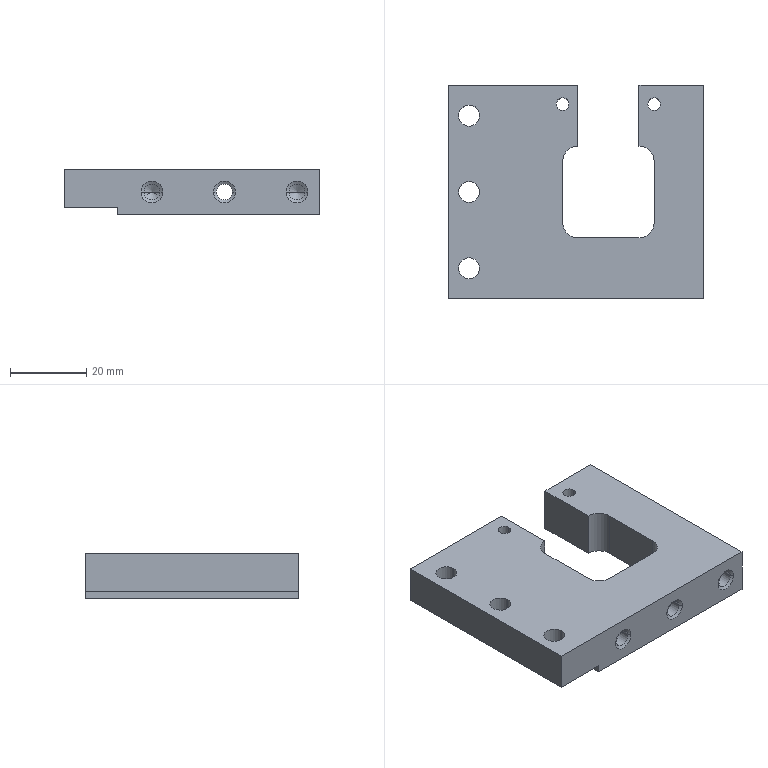Part | NX | 1 solid | 48 faces | box 67 x 56 x 12 mm | volume 32065 mm3 | cylinder 20 | plane 14 | cone 14 | commonest cylinder face diameters 4.2 x6 5.5 x6 3.3 x4 8 x4
STEP:
#1=CARTESIAN_POINT('',(480.1,203.33,-200.53));
#2=VERTEX_POINT('',#1);
#3=CARTESIAN_POINT('',(497.1,203.33,-200.53));
#4=VERTEX_POINT('',#3);
#5=CARTESIAN_POINT('',(435.607,203.33,-200.53));
#6=DIRECTION('',(1.,0.,0.));
#7=VECTOR('',#6,1000.);
#8=LINE('',#5,#7);
#9=EDGE_CURVE('',#2,#4,#8,.T.);
#10=ORIENTED_EDGE('',*,*,#9,.F.);
#11=CARTESIAN_POINT('',(480.1,203.33,-188.53));
#12=VERTEX_POINT('',#11);
#13=CARTESIAN_POINT('',(480.1,203.33,-198.53));
#14=DIRECTION('',(0.,0.,1.));
#15=VECTOR('',#14,1000.);
#16=LINE('',#13,#15);
#17=EDGE_CURVE('',#2,#12,#16,.T.);
#18=ORIENTED_EDGE('',*,*,#17,.T.);
#19=CARTESIAN_POINT('',(497.1,203.33,-188.53));
#20=VERTEX_POINT('',#19);
#21=CARTESIAN_POINT('',(435.607,203.33,-188.53));
#22=DIRECTION('',(-1.,0.,0.));
#23=VECTOR('',#22,1000.);
#24=LINE('',#21,#23);
#25=EDGE_CURVE('',#20,#12,#24,.T.);
#26=ORIENTED_EDGE('',*,*,#25,.F.);
#27=CARTESIAN_POINT('',(497.1,203.33,-198.53));
#28=DIRECTION('',(0.,0.,1.));
#29=VECTOR('',#28,1000.);
#30=LINE('',#27,#29);
#31=EDGE_CURVE('',#4,#20,#30,.T.);
#32=ORIENTED_EDGE('',*,*,#31,.F.);
#33=EDGE_LOOP('',(#10,#18,#26,#32));
#34=FACE_BOUND('',#33,.T.);
#35=CARTESIAN_POINT('',(430.1,203.33,-198.53));
#36=DIRECTION('',(0.,1.,0.));
#37=DIRECTION('',(1.,0.,0.));
#38=AXIS2_PLACEMENT_3D('',#35,#36,#37);
#39=PLANE('',#38);
#40=ADVANCED_FACE('',(#34),#39,.T.);
#41=CARTESIAN_POINT('',(430.1,147.33,-198.53));
#42=VERTEX_POINT('',#41);
#43=CARTESIAN_POINT('',(444.1,147.33,-198.53));
#44=VERTEX_POINT('',#43);
#45=CARTESIAN_POINT('',(435.607,147.33,-198.53));
#46=DIRECTION('',(1.,0.,0.));
#47=VECTOR('',#46,1000.);
#48=LINE('',#45,#47);
#49=EDGE_CURVE('',#42,#44,#48,.T.);
#50=ORIENTED_EDGE('',*,*,#49,.T.);
#51=CARTESIAN_POINT('',(444.1,147.33,-200.53));
#52=VERTEX_POINT('',#51);
#53=CARTESIAN_POINT('',(444.1,147.33,-198.53));
#54=DIRECTION('',(0.,0.,1.));
#55=VECTOR('',#54,1000.);
#56=LINE('',#53,#55);
#57=EDGE_CURVE('',#52,#44,#56,.T.);
#58=ORIENTED_EDGE('',*,*,#57,.F.);
#59=CARTESIAN_POINT('',(497.1,147.33,-200.53));
#60=VERTEX_POINT('',#59);
#61=CARTESIAN_POINT('',(435.607,147.33,-200.53));
#62=DIRECTION('',(-1.,0.,0.));
#63=VECTOR('',#62,1000.);
#64=LINE('',#61,#63);
#65=EDGE_CURVE('',#60,#52,#64,.T.);
#66=ORIENTED_EDGE('',*,*,#65,.F.);
#67=CARTESIAN_POINT('',(497.1,147.33,-188.53));
#68=VERTEX_POINT('',#67);
#69=CARTESIAN_POINT('',(497.1,147.33,-198.53));
#70=DIRECTION('',(0.,0.,1.));
#71=VECTOR('',#70,1000.);
#72=LINE('',#69,#71);
#73=EDGE_CURVE('',#60,#68,#72,.T.);
#74=ORIENTED_EDGE('',*,*,#73,.T.);
#75=CARTESIAN_POINT('',(430.1,147.33,-188.53));
#76=VERTEX_POINT('',#75);
#77=CARTESIAN_POINT('',(435.607,147.33,-188.53));
#78=DIRECTION('',(1.,0.,0.));
#79=VECTOR('',#78,1000.);
#80=LINE('',#77,#79);
#81=EDGE_CURVE('',#76,#68,#80,.T.);
#82=ORIENTED_EDGE('',*,*,#81,.F.);
#83=CARTESIAN_POINT('',(430.1,147.33,-198.53));
#84=DIRECTION('',(0.,0.,-1.));
#85=VECTOR('',#84,1000.);
#86=LINE('',#83,#85);
#87=EDGE_CURVE('',#76,#42,#86,.T.);
#88=ORIENTED_EDGE('',*,*,#87,.T.);
#89=EDGE_LOOP('',(#50,#58,#66,#74,#82,#88));
#90=FACE_BOUND('',#89,.T.);
#91=CARTESIAN_POINT('',(469.24,147.33,-194.53));
#92=VERTEX_POINT('',#91);
#93=CARTESIAN_POINT('',(474.96,147.33,-194.53));
#94=VERTEX_POINT('',#93);
#95=CARTESIAN_POINT('',(472.1,147.33,-194.53));
#96=DIRECTION('',(0.,-1.,0.));
#97=DIRECTION('',(-1.,0.,0.));
#98=AXIS2_PLACEMENT_3D('',#95,#96,#97);
#99=CIRCLE('',#98,2.86);
#100=EDGE_CURVE('',#92,#94,#99,.T.);
#101=ORIENTED_EDGE('',*,*,#100,.F.);
#102=CARTESIAN_POINT('',(472.1,147.33,-194.53));
#103=DIRECTION('',(0.,-1.,0.));
#104=DIRECTION('',(-1.,0.,0.));
#105=AXIS2_PLACEMENT_3D('',#102,#103,#104);
#106=CIRCLE('',#105,2.86);
#107=EDGE_CURVE('',#94,#92,#106,.T.);
#108=ORIENTED_EDGE('',*,*,#107,.F.);
#109=EDGE_LOOP('',(#101,#108));
#110=FACE_BOUND('',#109,.T.);
#111=CARTESIAN_POINT('',(455.96,147.33,-194.53));
#112=VERTEX_POINT('',#111);
#113=CARTESIAN_POINT('',(450.24,147.33,-194.53));
#114=VERTEX_POINT('',#113);
#115=CARTESIAN_POINT('',(453.1,147.33,-194.53));
#116=DIRECTION('',(0.,-1.,0.));
#117=DIRECTION('',(-1.,0.,0.));
#118=AXIS2_PLACEMENT_3D('',#115,#116,#117);
#119=CIRCLE('',#118,2.86);
#120=EDGE_CURVE('',#112,#114,#119,.T.);
#121=ORIENTED_EDGE('',*,*,#120,.F.);
#122=CARTESIAN_POINT('',(453.1,147.33,-194.53));
#123=DIRECTION('',(0.,-1.,0.));
#124=DIRECTION('',(-1.,0.,0.));
#125=AXIS2_PLACEMENT_3D('',#122,#123,#124);
#126=CIRCLE('',#125,2.86);
#127=EDGE_CURVE('',#114,#112,#126,.T.);
#128=ORIENTED_EDGE('',*,*,#127,.F.);
#129=EDGE_LOOP('',(#121,#128));
#130=FACE_BOUND('',#129,.T.);
#131=CARTESIAN_POINT('',(488.24,147.33,-194.53));
#132=VERTEX_POINT('',#131);
#133=CARTESIAN_POINT('',(493.96,147.33,-194.53));
#134=VERTEX_POINT('',#133);
#135=CARTESIAN_POINT('',(491.1,147.33,-194.53));
#136=DIRECTION('',(0.,-1.,0.));
#137=DIRECTION('',(-1.,0.,0.));
#138=AXIS2_PLACEMENT_3D('',#135,#136,#137);
#139=CIRCLE('',#138,2.86);
#140=EDGE_CURVE('',#132,#134,#139,.T.);
#141=ORIENTED_EDGE('',*,*,#140,.F.);
#142=CARTESIAN_POINT('',(491.1,147.33,-194.53));
#143=DIRECTION('',(0.,-1.,0.));
#144=DIRECTION('',(-1.,0.,0.));
#145=AXIS2_PLACEMENT_3D('',#142,#143,#144);
#146=CIRCLE('',#145,2.86);
#147=EDGE_CURVE('',#134,#132,#146,.T.);
#148=ORIENTED_EDGE('',*,*,#147,.F.);
#149=EDGE_LOOP('',(#141,#148));
#150=FACE_BOUND('',#149,.T.);
#151=CARTESIAN_POINT('',(444.1,147.33,-198.53));
#152=DIRECTION('',(0.,-1.,0.));
#153=DIRECTION('',(0.,0.,-1.));
#154=AXIS2_PLACEMENT_3D('',#151,#152,#153);
#155=PLANE('',#154);
#156=ADVANCED_FACE('',(#90,#110,#130,#150),#155,.T.);
#157=CARTESIAN_POINT('',(430.1,203.33,-198.53));
#158=VERTEX_POINT('',#157);
#159=CARTESIAN_POINT('',(430.1,236.208,-198.53));
#160=DIRECTION('',(0.,1.,0.));
#161=VECTOR('',#160,1000.);
#162=LINE('',#159,#161);
#163=EDGE_CURVE('',#42,#158,#162,.T.);
#164=ORIENTED_EDGE('',*,*,#163,.F.);
#165=ORIENTED_EDGE('',*,*,#87,.F.);
#166=CARTESIAN_POINT('',(430.1,203.33,-188.53));
#167=VERTEX_POINT('',#166);
#168=CARTESIAN_POINT('',(430.1,236.208,-188.53));
#169=DIRECTION('',(0.,-1.,0.));
#170=VECTOR('',#169,1000.);
#171=LINE('',#168,#170);
#172=EDGE_CURVE('',#167,#76,#171,.T.);
#173=ORIENTED_EDGE('',*,*,#172,.F.);
#174=CARTESIAN_POINT('',(430.1,203.33,-198.53));
#175=DIRECTION('',(0.,0.,-1.));
#176=VECTOR('',#175,1000.);
#177=LINE('',#174,#176);
#178=EDGE_CURVE('',#167,#158,#177,.T.);
#179=ORIENTED_EDGE('',*,*,#178,.T.);
#180=EDGE_LOOP('',(#164,#165,#173,#179));
#181=FACE_BOUND('',#180,.T.);
#182=CARTESIAN_POINT('',(430.1,145.33,-198.53));
#183=DIRECTION('',(-1.,0.,0.));
#184=DIRECTION('',(0.,0.,1.));
#185=AXIS2_PLACEMENT_3D('',#182,#183,#184);
#186=PLANE('',#185);
#187=ADVANCED_FACE('',(#181),#186,.T.);
#188=CARTESIAN_POINT('',(497.1,236.208,-200.53));
#189=DIRECTION('',(0.,-1.,0.));
#190=VECTOR('',#189,1000.);
#191=LINE('',#188,#190);
#192=EDGE_CURVE('',#4,#60,#191,.T.);
#193=ORIENTED_EDGE('',*,*,#192,.F.);
#194=ORIENTED_EDGE('',*,*,#31,.T.);
#195=CARTESIAN_POINT('',(497.1,236.208,-188.53));
#196=DIRECTION('',(0.,1.,0.));
#197=VECTOR('',#196,1000.);
#198=LINE('',#195,#197);
#199=EDGE_CURVE('',#68,#20,#198,.T.);
#200=ORIENTED_EDGE('',*,*,#199,.F.);
#201=ORIENTED_EDGE('',*,*,#73,.F.);
#202=EDGE_LOOP('',(#193,#194,#200,#201));
#203=FACE_BOUND('',#202,.T.);
#204=CARTESIAN_POINT('',(497.1,139.33,-198.528));
#205=DIRECTION('',(1.,0.,0.));
#206=DIRECTION('',(0.,-1.,0.));
#207=AXIS2_PLACEMENT_3D('',#204,#205,#206);
#208=PLANE('',#207);
#209=ADVANCED_FACE('',(#203),#208,.T.);
#210=ORIENTED_EDGE('',*,*,#49,.F.);
#211=ORIENTED_EDGE('',*,*,#163,.T.);
#212=CARTESIAN_POINT('',(444.1,203.33,-198.53));
#213=VERTEX_POINT('',#212);
#214=CARTESIAN_POINT('',(435.607,203.33,-198.53));
#215=DIRECTION('',(1.,0.,0.));
#216=VECTOR('',#215,1000.);
#217=LINE('',#214,#216);
#218=EDGE_CURVE('',#158,#213,#217,.T.);
#219=ORIENTED_EDGE('',*,*,#218,.T.);
#220=CARTESIAN_POINT('',(444.1,236.208,-198.53));
#221=DIRECTION('',(0.,-1.,0.));
#222=VECTOR('',#221,1000.);
#223=LINE('',#220,#222);
#224=EDGE_CURVE('',#213,#44,#223,.T.);
#225=ORIENTED_EDGE('',*,*,#224,.T.);
#226=EDGE_LOOP('',(#210,#211,#219,#225));
#227=FACE_BOUND('',#226,.T.);
#228=CARTESIAN_POINT('',(438.35,155.33,-198.53));
#229=VERTEX_POINT('',#228);
#230=CARTESIAN_POINT('',(432.85,155.33,-198.53));
#231=VERTEX_POINT('',#230);
#232=CARTESIAN_POINT('',(435.6,155.33,-198.53));
#233=DIRECTION('',(0.,0.,1.));
#234=DIRECTION('',(1.,0.,0.));
#235=AXIS2_PLACEMENT_3D('',#232,#233,#234);
#236=CIRCLE('',#235,2.75);
#237=EDGE_CURVE('',#229,#231,#236,.T.);
#238=ORIENTED_EDGE('',*,*,#237,.T.);
#239=CARTESIAN_POINT('',(435.6,155.33,-198.53));
#240=DIRECTION('',(0.,0.,1.));
#241=DIRECTION('',(1.,0.,0.));
#242=AXIS2_PLACEMENT_3D('',#239,#240,#241);
#243=CIRCLE('',#242,2.75);
#244=EDGE_CURVE('',#231,#229,#243,.T.);
#245=ORIENTED_EDGE('',*,*,#244,.T.);
#246=EDGE_LOOP('',(#238,#245));
#247=FACE_BOUND('',#246,.T.);
#248=CARTESIAN_POINT('',(438.35,195.33,-198.53));
#249=VERTEX_POINT('',#248);
#250=CARTESIAN_POINT('',(432.85,195.33,-198.53));
#251=VERTEX_POINT('',#250);
#252=CARTESIAN_POINT('',(435.6,195.33,-198.53));
#253=DIRECTION('',(0.,0.,1.));
#254=DIRECTION('',(1.,0.,0.));
#255=AXIS2_PLACEMENT_3D('',#252,#253,#254);
#256=CIRCLE('',#255,2.75);
#257=EDGE_CURVE('',#249,#251,#256,.T.);
#258=ORIENTED_EDGE('',*,*,#257,.T.);
#259=CARTESIAN_POINT('',(435.6,195.33,-198.53));
#260=DIRECTION('',(0.,0.,1.));
#261=DIRECTION('',(1.,0.,0.));
#262=AXIS2_PLACEMENT_3D('',#259,#260,#261);
#263=CIRCLE('',#262,2.75);
#264=EDGE_CURVE('',#251,#249,#263,.T.);
#265=ORIENTED_EDGE('',*,*,#264,.T.);
#266=EDGE_LOOP('',(#258,#265));
#267=FACE_BOUND('',#266,.T.);
#268=CARTESIAN_POINT('',(438.35,175.33,-198.53));
#269=VERTEX_POINT('',#268);
#270=CARTESIAN_POINT('',(432.85,175.33,-198.53));
#271=VERTEX_POINT('',#270);
#272=CARTESIAN_POINT('',(435.6,175.33,-198.53));
#273=DIRECTION('',(0.,0.,1.));
#274=DIRECTION('',(1.,0.,0.));
#275=AXIS2_PLACEMENT_3D('',#272,#273,#274);
#276=CIRCLE('',#275,2.75);
#277=EDGE_CURVE('',#269,#271,#276,.T.);
#278=ORIENTED_EDGE('',*,*,#277,.T.);
#279=CARTESIAN_POINT('',(435.6,175.33,-198.53));
#280=DIRECTION('',(0.,0.,1.));
#281=DIRECTION('',(1.,0.,0.));
#282=AXIS2_PLACEMENT_3D('',#279,#280,#281);
#283=CIRCLE('',#282,2.75);
#284=EDGE_CURVE('',#271,#269,#283,.T.);
#285=ORIENTED_EDGE('',*,*,#284,.T.);
#286=EDGE_LOOP('',(#278,#285));
#287=FACE_BOUND('',#286,.T.);
#288=CARTESIAN_POINT('',(437.503,173.26,-198.53));
#289=DIRECTION('',(0.,0.,-1.));
#290=DIRECTION('',(0.,-1.,0.));
#291=AXIS2_PLACEMENT_3D('',#288,#289,#290);
#292=PLANE('',#291);
#293=ADVANCED_FACE('',(#227,#247,#267,#287),#292,.T.);
#294=ORIENTED_EDGE('',*,*,#57,.T.);
#295=ORIENTED_EDGE('',*,*,#224,.F.);
#296=CARTESIAN_POINT('',(444.1,203.33,-200.53));
#297=VERTEX_POINT('',#296);
#298=CARTESIAN_POINT('',(444.1,203.33,-198.53));
#299=DIRECTION('',(0.,0.,1.));
#300=VECTOR('',#299,1000.);
#301=LINE('',#298,#300);
#302=EDGE_CURVE('',#297,#213,#301,.T.);
#303=ORIENTED_EDGE('',*,*,#302,.F.);
#304=CARTESIAN_POINT('',(444.1,236.208,-200.53));
#305=DIRECTION('',(0.,-1.,0.));
#306=VECTOR('',#305,1000.);
#307=LINE('',#304,#306);
#308=EDGE_CURVE('',#297,#52,#307,.T.);
#309=ORIENTED_EDGE('',*,*,#308,.T.);
#310=EDGE_LOOP('',(#294,#295,#303,#309));
#311=FACE_BOUND('',#310,.T.);
#312=CARTESIAN_POINT('',(444.1,197.33,-200.53));
#313=DIRECTION('',(1.,0.,0.));
#314=DIRECTION('',(0.,1.,0.));
#315=AXIS2_PLACEMENT_3D('',#312,#313,#314);
#316=PLANE('',#315);
#317=ADVANCED_FACE('',(#311),#316,.F.);
#318=CARTESIAN_POINT('',(474.2,163.33,-194.53));
#319=VERTEX_POINT('',#318);
#320=CARTESIAN_POINT('',(470.,163.33,-194.53));
#321=VERTEX_POINT('',#320);
#322=CARTESIAN_POINT('',(472.1,163.33,-194.53));
#323=DIRECTION('',(0.,-1.,0.));
#324=DIRECTION('',(-1.,0.,0.));
#325=AXIS2_PLACEMENT_3D('',#322,#323,#324);
#326=CIRCLE('',#325,2.1);
#327=EDGE_CURVE('',#319,#321,#326,.T.);
#328=ORIENTED_EDGE('',*,*,#327,.F.);
#329=CARTESIAN_POINT('',(474.2,147.769,-194.53));
#330=VERTEX_POINT('',#329);
#331=CARTESIAN_POINT('',(474.2,147.33,-194.53));
#332=DIRECTION('',(0.,-1.,0.));
#333=VECTOR('',#332,1000.);
#334=LINE('',#331,#333);
#335=EDGE_CURVE('',#330,#319,#334,.F.);
#336=ORIENTED_EDGE('',*,*,#335,.F.);
#337=CARTESIAN_POINT('',(470.,147.769,-194.53));
#338=VERTEX_POINT('',#337);
#339=CARTESIAN_POINT('',(472.1,147.769,-194.53));
#340=DIRECTION('',(0.,-1.,0.));
#341=DIRECTION('',(-1.,0.,0.));
#342=AXIS2_PLACEMENT_3D('',#339,#340,#341);
#343=CIRCLE('',#342,2.1);
#344=EDGE_CURVE('',#330,#338,#343,.T.);
#345=ORIENTED_EDGE('',*,*,#344,.T.);
#346=CARTESIAN_POINT('',(470.,147.33,-194.53));
#347=DIRECTION('',(0.,-1.,0.));
#348=VECTOR('',#347,1000.);
#349=LINE('',#346,#348);
#350=EDGE_CURVE('',#338,#321,#349,.F.);
#351=ORIENTED_EDGE('',*,*,#350,.T.);
#352=EDGE_LOOP('',(#328,#336,#345,#351));
#353=FACE_BOUND('',#352,.T.);
#354=CARTESIAN_POINT('',(472.1,147.33,-194.53));
#355=DIRECTION('',(0.,-1.,0.));
#356=DIRECTION('',(-1.,0.,0.));
#357=AXIS2_PLACEMENT_3D('',#354,#355,#356);
#358=CYLINDRICAL_SURFACE('',#357,2.1);
#359=ADVANCED_FACE('',(#353),#358,.F.);
#360=CARTESIAN_POINT('',(464.1,203.33,-200.53));
#361=VERTEX_POINT('',#360);
#362=CARTESIAN_POINT('',(435.607,203.33,-200.53));
#363=DIRECTION('',(1.,0.,0.));
#364=VECTOR('',#363,1000.);
#365=LINE('',#362,#364);
#366=EDGE_CURVE('',#297,#361,#365,.T.);
#367=ORIENTED_EDGE('',*,*,#366,.F.);
#368=ORIENTED_EDGE('',*,*,#302,.T.);
#369=ORIENTED_EDGE('',*,*,#218,.F.);
#370=ORIENTED_EDGE('',*,*,#178,.F.);
#371=CARTESIAN_POINT('',(464.1,203.33,-188.53));
#372=VERTEX_POINT('',#371);
#373=CARTESIAN_POINT('',(435.607,203.33,-188.53));
#374=DIRECTION('',(-1.,0.,0.));
#375=VECTOR('',#374,1000.);
#376=LINE('',#373,#375);
#377=EDGE_CURVE('',#372,#167,#376,.T.);
#378=ORIENTED_EDGE('',*,*,#377,.F.);
#379=CARTESIAN_POINT('',(464.1,203.33,-198.53));
#380=DIRECTION('',(0.,0.,-1.));
#381=VECTOR('',#380,1000.);
#382=LINE('',#379,#381);
#383=EDGE_CURVE('',#372,#361,#382,.T.);
#384=ORIENTED_EDGE('',*,*,#383,.T.);
#385=EDGE_LOOP('',(#367,#368,#369,#370,#378,#384));
#386=FACE_BOUND('',#385,.T.);
#387=CARTESIAN_POINT('',(430.1,203.33,-198.53));
#388=DIRECTION('',(0.,1.,0.));
#389=DIRECTION('',(1.,0.,0.));
#390=AXIS2_PLACEMENT_3D('',#387,#388,#389);
#391=PLANE('',#390);
#392=ADVANCED_FACE('',(#386),#391,.T.);
#393=ORIENTED_EDGE('',*,*,#25,.T.);
#394=CARTESIAN_POINT('',(480.1,187.33,-188.53));
#395=VERTEX_POINT('',#394);
#396=CARTESIAN_POINT('',(480.1,236.208,-188.53));
#397=DIRECTION('',(0.,-1.,0.));
#398=VECTOR('',#397,1000.);
#399=LINE('',#396,#398);
#400=EDGE_CURVE('',#12,#395,#399,.T.);
#401=ORIENTED_EDGE('',*,*,#400,.T.);
#402=CARTESIAN_POINT('',(484.1,183.33,-188.53));
#403=VERTEX_POINT('',#402);
#404=CARTESIAN_POINT('',(480.1,183.33,-188.53));
#405=DIRECTION('',(0.,0.,-1.));
#406=DIRECTION('',(-1.,0.,0.));
#407=AXIS2_PLACEMENT_3D('',#404,#405,#406);
#408=CIRCLE('',#407,4.);
#409=EDGE_CURVE('',#395,#403,#408,.T.);
#410=ORIENTED_EDGE('',*,*,#409,.T.);
#411=CARTESIAN_POINT('',(484.1,167.33,-188.53));
#412=VERTEX_POINT('',#411);
#413=CARTESIAN_POINT('',(484.1,236.208,-188.53));
#414=DIRECTION('',(0.,1.,0.));
#415=VECTOR('',#414,1000.);
#416=LINE('',#413,#415);
#417=EDGE_CURVE('',#412,#403,#416,.T.);
#418=ORIENTED_EDGE('',*,*,#417,.F.);
#419=CARTESIAN_POINT('',(480.1,163.33,-188.53));
#420=VERTEX_POINT('',#419);
#421=CARTESIAN_POINT('',(480.1,167.33,-188.53));
#422=DIRECTION('',(0.,0.,-1.));
#423=DIRECTION('',(-1.,0.,0.));
#424=AXIS2_PLACEMENT_3D('',#421,#422,#423);
#425=CIRCLE('',#424,4.);
#426=EDGE_CURVE('',#412,#420,#425,.T.);
#427=ORIENTED_EDGE('',*,*,#426,.T.);
#428=CARTESIAN_POINT('',(464.1,163.33,-188.53));
#429=VERTEX_POINT('',#428);
#430=CARTESIAN_POINT('',(435.607,163.33,-188.53));
#431=DIRECTION('',(-1.,0.,0.));
#432=VECTOR('',#431,1000.);
#433=LINE('',#430,#432);
#434=EDGE_CURVE('',#420,#429,#433,.T.);
#435=ORIENTED_EDGE('',*,*,#434,.T.);
#436=CARTESIAN_POINT('',(460.1,167.33,-188.53));
#437=VERTEX_POINT('',#436);
#438=CARTESIAN_POINT('',(464.1,167.33,-188.53));
#439=DIRECTION('',(0.,0.,1.));
#440=DIRECTION('',(1.,0.,0.));
#441=AXIS2_PLACEMENT_3D('',#438,#439,#440);
#442=CIRCLE('',#441,4.);
#443=EDGE_CURVE('',#437,#429,#442,.T.);
#444=ORIENTED_EDGE('',*,*,#443,.F.);
#445=CARTESIAN_POINT('',(460.1,183.33,-188.53));
#446=VERTEX_POINT('',#445);
#447=CARTESIAN_POINT('',(460.1,236.208,-188.53));
#448=DIRECTION('',(0.,-1.,0.));
#449=VECTOR('',#448,1000.);
#450=LINE('',#447,#449);
#451=EDGE_CURVE('',#446,#437,#450,.T.);
#452=ORIENTED_EDGE('',*,*,#451,.F.);
#453=CARTESIAN_POINT('',(464.1,187.33,-188.53));
#454=VERTEX_POINT('',#453);
#455=CARTESIAN_POINT('',(464.1,183.33,-188.53));
#456=DIRECTION('',(0.,0.,1.));
#457=DIRECTION('',(1.,0.,0.));
#458=AXIS2_PLACEMENT_3D('',#455,#456,#457);
#459=CIRCLE('',#458,4.);
#460=EDGE_CURVE('',#454,#446,#459,.T.);
#461=ORIENTED_EDGE('',*,*,#460,.F.);
#462=CARTESIAN_POINT('',(464.1,236.208,-188.53));
#463=DIRECTION('',(0.,1.,0.));
#464=VECTOR('',#463,1000.);
#465=LINE('',#462,#464);
#466=EDGE_CURVE('',#454,#372,#465,.T.);
#467=ORIENTED_EDGE('',*,*,#466,.T.);
#468=ORIENTED_EDGE('',*,*,#377,.T.);
#469=ORIENTED_EDGE('',*,*,#172,.T.);
#470=ORIENTED_EDGE('',*,*,#81,.T.);
#471=ORIENTED_EDGE('',*,*,#199,.T.);
#472=EDGE_LOOP('',(#393,#401,#410,#418,#427,#435,#444,#452,#461,#467,#468,#469,#470,#471));
#473=FACE_BOUND('',#472,.T.);
#474=CARTESIAN_POINT('',(461.75,198.33,-188.53));
#475=VERTEX_POINT('',#474);
#476=CARTESIAN_POINT('',(458.45,198.33,-188.53));
#477=VERTEX_POINT('',#476);
#478=CARTESIAN_POINT('',(460.1,198.33,-188.53));
#479=DIRECTION('',(0.,0.,-1.));
#480=DIRECTION('',(-1.,0.,0.));
#481=AXIS2_PLACEMENT_3D('',#478,#479,#480);
#482=CIRCLE('',#481,1.65);
#483=EDGE_CURVE('',#475,#477,#482,.T.);
#484=ORIENTED_EDGE('',*,*,#483,.T.);
#485=CARTESIAN_POINT('',(460.1,198.33,-188.53));
#486=DIRECTION('',(0.,0.,-1.));
#487=DIRECTION('',(-1.,0.,0.));
#488=AXIS2_PLACEMENT_3D('',#485,#486,#487);
#489=CIRCLE('',#488,1.65);
#490=EDGE_CURVE('',#477,#475,#489,.T.);
#491=ORIENTED_EDGE('',*,*,#490,.T.);
#492=EDGE_LOOP('',(#484,#491));
#493=FACE_BOUND('',#492,.T.);
#494=CARTESIAN_POINT('',(485.75,198.33,-188.53));
#495=VERTEX_POINT('',#494);
#496=CARTESIAN_POINT('',(482.45,198.33,-188.53));
#497=VERTEX_POINT('',#496);
#498=CARTESIAN_POINT('',(484.1,198.33,-188.53));
#499=DIRECTION('',(0.,0.,-1.));
#500=DIRECTION('',(-1.,0.,0.));
#501=AXIS2_PLACEMENT_3D('',#498,#499,#500);
#502=CIRCLE('',#501,1.65);
#503=EDGE_CURVE('',#495,#497,#502,.T.);
#504=ORIENTED_EDGE('',*,*,#503,.T.);
#505=CARTESIAN_POINT('',(484.1,198.33,-188.53));
#506=DIRECTION('',(0.,0.,-1.));
#507=DIRECTION('',(-1.,0.,0.));
#508=AXIS2_PLACEMENT_3D('',#505,#506,#507);
#509=CIRCLE('',#508,1.65);
#510=EDGE_CURVE('',#497,#495,#509,.T.);
#511=ORIENTED_EDGE('',*,*,#510,.T.);
#512=EDGE_LOOP('',(#504,#511));
#513=FACE_BOUND('',#512,.T.);
#514=CARTESIAN_POINT('',(438.35,175.33,-188.53));
#515=VERTEX_POINT('',#514);
#516=CARTESIAN_POINT('',(432.85,175.33,-188.53));
#517=VERTEX_POINT('',#516);
#518=CARTESIAN_POINT('',(435.6,175.33,-188.53));
#519=DIRECTION('',(0.,0.,1.));
#520=DIRECTION('',(1.,0.,0.));
#521=AXIS2_PLACEMENT_3D('',#518,#519,#520);
#522=CIRCLE('',#521,2.75);
#523=EDGE_CURVE('',#515,#517,#522,.T.);
#524=ORIENTED_EDGE('',*,*,#523,.F.);
#525=CARTESIAN_POINT('',(435.6,175.33,-188.53));
#526=DIRECTION('',(0.,0.,1.));
#527=DIRECTION('',(1.,0.,0.));
#528=AXIS2_PLACEMENT_3D('',#525,#526,#527);
#529=CIRCLE('',#528,2.75);
#530=EDGE_CURVE('',#517,#515,#529,.T.);
#531=ORIENTED_EDGE('',*,*,#530,.F.);
#532=EDGE_LOOP('',(#524,#531));
#533=FACE_BOUND('',#532,.T.);
#534=CARTESIAN_POINT('',(438.35,195.33,-188.53));
#535=VERTEX_POINT('',#534);
#536=CARTESIAN_POINT('',(432.85,195.33,-188.53));
#537=VERTEX_POINT('',#536);
#538=CARTESIAN_POINT('',(435.6,195.33,-188.53));
#539=DIRECTION('',(0.,0.,1.));
#540=DIRECTION('',(1.,0.,0.));
#541=AXIS2_PLACEMENT_3D('',#538,#539,#540);
#542=CIRCLE('',#541,2.75);
#543=EDGE_CURVE('',#535,#537,#542,.T.);
#544=ORIENTED_EDGE('',*,*,#543,.F.);
#545=CARTESIAN_POINT('',(435.6,195.33,-188.53));
#546=DIRECTION('',(0.,0.,1.));
#547=DIRECTION('',(1.,0.,0.));
#548=AXIS2_PLACEMENT_3D('',#545,#546,#547);
#549=CIRCLE('',#548,2.75);
#550=EDGE_CURVE('',#537,#535,#549,.T.);
#551=ORIENTED_EDGE('',*,*,#550,.F.);
#552=EDGE_LOOP('',(#544,#551));
#553=FACE_BOUND('',#552,.T.);
#554=CARTESIAN_POINT('',(438.35,155.33,-188.53));
#555=VERTEX_POINT('',#554);
#556=CARTESIAN_POINT('',(432.85,155.33,-188.53));
#557=VERTEX_POINT('',#556);
#558=CARTESIAN_POINT('',(435.6,155.33,-188.53));
#559=DIRECTION('',(0.,0.,1.));
#560=DIRECTION('',(1.,0.,0.));
#561=AXIS2_PLACEMENT_3D('',#558,#559,#560);
#562=CIRCLE('',#561,2.75);
#563=EDGE_CURVE('',#555,#557,#562,.T.);
#564=ORIENTED_EDGE('',*,*,#563,.F.);
#565=CARTESIAN_POINT('',(435.6,155.33,-188.53));
#566=DIRECTION('',(0.,0.,1.));
#567=DIRECTION('',(1.,0.,0.));
#568=AXIS2_PLACEMENT_3D('',#565,#566,#567);
#569=CIRCLE('',#568,2.75);
#570=EDGE_CURVE('',#557,#555,#569,.T.);
#571=ORIENTED_EDGE('',*,*,#570,.F.);
#572=EDGE_LOOP('',(#564,#571));
#573=FACE_BOUND('',#572,.T.);
#574=CARTESIAN_POINT('',(484.1,203.33,-188.53));
#575=DIRECTION('',(0.,0.,1.));
#576=DIRECTION('',(1.,0.,0.));
#577=AXIS2_PLACEMENT_3D('',#574,#575,#576);
#578=PLANE('',#577);
#579=ADVANCED_FACE('',(#473,#493,#513,#533,#553,#573),#578,.T.);
#580=ORIENTED_EDGE('',*,*,#344,.F.);
#581=CARTESIAN_POINT('',(474.2,147.769,-194.53));
#582=DIRECTION('',(0.866,-0.5,0.));
#583=VECTOR('',#582,1000.);
#584=LINE('',#581,#583);
#585=EDGE_CURVE('',#330,#94,#584,.T.);
#586=ORIENTED_EDGE('',*,*,#585,.T.);
#587=ORIENTED_EDGE('',*,*,#107,.T.);
#588=CARTESIAN_POINT('',(470.,147.769,-194.53));
#589=DIRECTION('',(-0.866,-0.5,0.));
#590=VECTOR('',#589,1000.);
#591=LINE('',#588,#590);
#592=EDGE_CURVE('',#338,#92,#591,.T.);
#593=ORIENTED_EDGE('',*,*,#592,.F.);
#594=EDGE_LOOP('',(#580,#586,#587,#593));
#595=FACE_BOUND('',#594,.T.);
#596=CARTESIAN_POINT('',(472.1,147.769,-194.53));
#597=DIRECTION('',(0.,-1.,0.));
#598=DIRECTION('',(-1.,0.,0.));
#599=AXIS2_PLACEMENT_3D('',#596,#597,#598);
#600=CONICAL_SURFACE('',#599,2.1,1.047);
#601=ADVANCED_FACE('',(#595),#600,.F.);
#602=CARTESIAN_POINT('',(451.,147.769,-194.53));
#603=VERTEX_POINT('',#602);
#604=CARTESIAN_POINT('',(455.2,147.769,-194.53));
#605=VERTEX_POINT('',#604);
#606=CARTESIAN_POINT('',(453.1,147.769,-194.53));
#607=DIRECTION('',(0.,-1.,0.));
#608=DIRECTION('',(-1.,0.,0.));
#609=AXIS2_PLACEMENT_3D('',#606,#607,#608);
#610=CIRCLE('',#609,2.1);
#611=EDGE_CURVE('',#603,#605,#610,.T.);
#612=ORIENTED_EDGE('',*,*,#611,.T.);
#613=CARTESIAN_POINT('',(455.2,162.13,-194.53));
#614=VERTEX_POINT('',#613);
#615=CARTESIAN_POINT('',(455.2,147.33,-194.53));
#616=DIRECTION('',(0.,-1.,0.));
#617=VECTOR('',#616,1000.);
#618=LINE('',#615,#617);
#619=EDGE_CURVE('',#605,#614,#618,.F.);
#620=ORIENTED_EDGE('',*,*,#619,.T.);
#621=CARTESIAN_POINT('',(451.,162.13,-194.53));
#622=VERTEX_POINT('',#621);
#623=CARTESIAN_POINT('',(453.1,162.13,-194.53));
#624=DIRECTION('',(0.,-1.,0.));
#625=DIRECTION('',(-1.,0.,0.));
#626=AXIS2_PLACEMENT_3D('',#623,#624,#625);
#627=CIRCLE('',#626,2.1);
#628=EDGE_CURVE('',#622,#614,#627,.T.);
#629=ORIENTED_EDGE('',*,*,#628,.F.);
#630=CARTESIAN_POINT('',(451.,147.33,-194.53));
#631=DIRECTION('',(0.,-1.,0.));
#632=VECTOR('',#631,1000.);
#633=LINE('',#630,#632);
#634=EDGE_CURVE('',#603,#622,#633,.F.);
#635=ORIENTED_EDGE('',*,*,#634,.F.);
#636=EDGE_LOOP('',(#612,#620,#629,#635));
#637=FACE_BOUND('',#636,.T.);
#638=CARTESIAN_POINT('',(453.1,147.33,-194.53));
#639=DIRECTION('',(0.,-1.,0.));
#640=DIRECTION('',(-1.,0.,0.));
#641=AXIS2_PLACEMENT_3D('',#638,#639,#640);
#642=CYLINDRICAL_SURFACE('',#641,2.1);
#643=ADVANCED_FACE('',(#637),#642,.F.);
#644=CARTESIAN_POINT('',(484.1,167.33,-200.53));
#645=VERTEX_POINT('',#644);
#646=CARTESIAN_POINT('',(484.1,167.33,-198.53));
#647=DIRECTION('',(0.,0.,-1.));
#648=VECTOR('',#647,1000.);
#649=LINE('',#646,#648);
#650=EDGE_CURVE('',#412,#645,#649,.T.);
#651=ORIENTED_EDGE('',*,*,#650,.T.);
#652=CARTESIAN_POINT('',(480.1,163.33,-200.53));
#653=VERTEX_POINT('',#652);
#654=CARTESIAN_POINT('',(480.1,167.33,-200.53));
#655=DIRECTION('',(0.,0.,-1.));
#656=DIRECTION('',(-1.,0.,0.));
#657=AXIS2_PLACEMENT_3D('',#654,#655,#656);
#658=CIRCLE('',#657,4.);
#659=EDGE_CURVE('',#645,#653,#658,.T.);
#660=ORIENTED_EDGE('',*,*,#659,.T.);
#661=CARTESIAN_POINT('',(480.1,163.33,-198.53));
#662=DIRECTION('',(0.,0.,-1.));
#663=VECTOR('',#662,1000.);
#664=LINE('',#661,#663);
#665=EDGE_CURVE('',#420,#653,#664,.T.);
#666=ORIENTED_EDGE('',*,*,#665,.F.);
#667=ORIENTED_EDGE('',*,*,#426,.F.);
#668=EDGE_LOOP('',(#651,#660,#666,#667));
#669=FACE_BOUND('',#668,.T.);
#670=CARTESIAN_POINT('',(480.1,167.33,-198.53));
#671=DIRECTION('',(0.,0.,-1.));
#672=DIRECTION('',(-1.,0.,0.));
#673=AXIS2_PLACEMENT_3D('',#670,#671,#672);
#674=CYLINDRICAL_SURFACE('',#673,4.);
#675=ADVANCED_FACE('',(#669),#674,.F.);
#676=CARTESIAN_POINT('',(453.1,163.392,-194.53));
#677=VERTEX_POINT('',#676);
#678=CARTESIAN_POINT('',(455.2,162.13,-194.53));
#679=DIRECTION('',(0.8572,-0.515,0.));
#680=VECTOR('',#679,1000.);
#681=LINE('',#678,#680);
#682=EDGE_CURVE('',#677,#614,#681,.T.);
#683=ORIENTED_EDGE('',*,*,#682,.T.);
#684=CARTESIAN_POINT('',(453.1,162.13,-194.53));
#685=DIRECTION('',(0.,-1.,0.));
#686=DIRECTION('',(-1.,0.,0.));
#687=AXIS2_PLACEMENT_3D('',#684,#685,#686);
#688=CIRCLE('',#687,2.1);
#689=EDGE_CURVE('',#614,#622,#688,.T.);
#690=ORIENTED_EDGE('',*,*,#689,.T.);
#691=CARTESIAN_POINT('',(451.,162.13,-194.53));
#692=DIRECTION('',(-0.8572,-0.515,0.));
#693=VECTOR('',#692,1000.);
#694=LINE('',#691,#693);
#695=EDGE_CURVE('',#677,#622,#694,.T.);
#696=ORIENTED_EDGE('',*,*,#695,.F.);
#697=EDGE_LOOP('',(#683,#690,#696));
#698=FACE_BOUND('',#697,.T.);
#699=CARTESIAN_POINT('',(453.1,162.13,-194.53));
#700=DIRECTION('',(0.,-1.,0.));
#701=DIRECTION('',(-1.,0.,0.));
#702=AXIS2_PLACEMENT_3D('',#699,#700,#701);
#703=CONICAL_SURFACE('',#702,2.1,1.03);
#704=ADVANCED_FACE('',(#698),#703,.F.);
#705=ORIENTED_EDGE('',*,*,#120,.T.);
#706=CARTESIAN_POINT('',(451.,147.769,-194.53));
#707=DIRECTION('',(-0.866,-0.5,0.));
#708=VECTOR('',#707,1000.);
#709=LINE('',#706,#708);
#710=EDGE_CURVE('',#114,#603,#709,.F.);
#711=ORIENTED_EDGE('',*,*,#710,.T.);
#712=CARTESIAN_POINT('',(453.1,147.769,-194.53));
#713=DIRECTION('',(0.,-1.,0.));
#714=DIRECTION('',(-1.,0.,0.));
#715=AXIS2_PLACEMENT_3D('',#712,#713,#714);
#716=CIRCLE('',#715,2.1);
#717=EDGE_CURVE('',#605,#603,#716,.T.);
#718=ORIENTED_EDGE('',*,*,#717,.F.);
#719=CARTESIAN_POINT('',(455.2,147.769,-194.53));
#720=DIRECTION('',(0.866,-0.5,0.));
#721=VECTOR('',#720,1000.);
#722=LINE('',#719,#721);
#723=EDGE_CURVE('',#112,#605,#722,.F.);
#724=ORIENTED_EDGE('',*,*,#723,.F.);
#725=EDGE_LOOP('',(#705,#711,#718,#724));
#726=FACE_BOUND('',#725,.T.);
#727=CARTESIAN_POINT('',(453.1,147.769,-194.53));
#728=DIRECTION('',(0.,-1.,0.));
#729=DIRECTION('',(-1.,0.,0.));
#730=AXIS2_PLACEMENT_3D('',#727,#728,#729);
#731=CONICAL_SURFACE('',#730,2.1,1.047);
#732=ADVANCED_FACE('',(#726),#731,.F.);
#733=CARTESIAN_POINT('',(489.,147.769,-194.53));
#734=VERTEX_POINT('',#733);
#735=CARTESIAN_POINT('',(493.2,147.769,-194.53));
#736=VERTEX_POINT('',#735);
#737=CARTESIAN_POINT('',(491.1,147.769,-194.53));
#738=DIRECTION('',(0.,-1.,0.));
#739=DIRECTION('',(-1.,0.,0.));
#740=AXIS2_PLACEMENT_3D('',#737,#738,#739);
#741=CIRCLE('',#740,2.1);
#742=EDGE_CURVE('',#734,#736,#741,.T.);
#743=ORIENTED_EDGE('',*,*,#742,.T.);
#744=CARTESIAN_POINT('',(493.2,162.13,-194.53));
#745=VERTEX_POINT('',#744);
#746=CARTESIAN_POINT('',(493.2,147.33,-194.53));
#747=DIRECTION('',(0.,-1.,0.));
#748=VECTOR('',#747,1000.);
#749=LINE('',#746,#748);
#750=EDGE_CURVE('',#745,#736,#749,.T.);
#751=ORIENTED_EDGE('',*,*,#750,.F.);
#752=CARTESIAN_POINT('',(489.,162.13,-194.53));
#753=VERTEX_POINT('',#752);
#754=CARTESIAN_POINT('',(491.1,162.13,-194.53));
#755=DIRECTION('',(0.,-1.,0.));
#756=DIRECTION('',(-1.,0.,0.));
#757=AXIS2_PLACEMENT_3D('',#754,#755,#756);
#758=CIRCLE('',#757,2.1);
#759=EDGE_CURVE('',#753,#745,#758,.T.);
#760=ORIENTED_EDGE('',*,*,#759,.F.);
#761=CARTESIAN_POINT('',(489.,147.33,-194.53));
#762=DIRECTION('',(0.,-1.,0.));
#763=VECTOR('',#762,1000.);
#764=LINE('',#761,#763);
#765=EDGE_CURVE('',#753,#734,#764,.T.);
#766=ORIENTED_EDGE('',*,*,#765,.T.);
#767=EDGE_LOOP('',(#743,#751,#760,#766));
#768=FACE_BOUND('',#767,.T.);
#769=CARTESIAN_POINT('',(491.1,147.33,-194.53));
#770=DIRECTION('',(0.,-1.,0.));
#771=DIRECTION('',(-1.,0.,0.));
#772=AXIS2_PLACEMENT_3D('',#769,#770,#771);
#773=CYLINDRICAL_SURFACE('',#772,2.1);
#774=ADVANCED_FACE('',(#768),#773,.F.);
#775=ORIENTED_EDGE('',*,*,#434,.F.);
#776=ORIENTED_EDGE('',*,*,#665,.T.);
#777=CARTESIAN_POINT('',(464.1,163.33,-200.53));
#778=VERTEX_POINT('',#777);
#779=CARTESIAN_POINT('',(435.607,163.33,-200.53));
#780=DIRECTION('',(1.,0.,0.));
#781=VECTOR('',#780,1000.);
#782=LINE('',#779,#781);
#783=EDGE_CURVE('',#778,#653,#782,.T.);
#784=ORIENTED_EDGE('',*,*,#783,.F.);
#785=CARTESIAN_POINT('',(464.1,163.33,-198.53));
#786=DIRECTION('',(0.,0.,1.));
#787=VECTOR('',#786,1000.);
#788=LINE('',#785,#787);
#789=EDGE_CURVE('',#778,#429,#788,.T.);
#790=ORIENTED_EDGE('',*,*,#789,.T.);
#791=EDGE_LOOP('',(#775,#776,#784,#790));
#792=FACE_BOUND('',#791,.T.);
#793=ORIENTED_EDGE('',*,*,#327,.T.);
#794=CARTESIAN_POINT('',(472.1,163.33,-194.53));
#795=DIRECTION('',(0.,-1.,0.));
#796=DIRECTION('',(-1.,0.,0.));
#797=AXIS2_PLACEMENT_3D('',#794,#795,#796);
#798=CIRCLE('',#797,2.1);
#799=EDGE_CURVE('',#321,#319,#798,.T.);
#800=ORIENTED_EDGE('',*,*,#799,.T.);
#801=EDGE_LOOP('',(#793,#800));
#802=FACE_BOUND('',#801,.T.);
#803=CARTESIAN_POINT('',(467.962,163.33,-193.196));
#804=DIRECTION('',(0.,1.,0.));
#805=DIRECTION('',(1.,0.,0.));
#806=AXIS2_PLACEMENT_3D('',#803,#804,#805);
#807=PLANE('',#806);
#808=ADVANCED_FACE('',(#792,#802),#807,.T.);
#809=CARTESIAN_POINT('',(491.1,163.392,-194.53));
#810=VERTEX_POINT('',#809);
#811=CARTESIAN_POINT('',(493.2,162.13,-194.53));
#812=DIRECTION('',(0.8572,-0.515,0.));
#813=VECTOR('',#812,1000.);
#814=LINE('',#811,#813);
#815=EDGE_CURVE('',#810,#745,#814,.T.);
#816=ORIENTED_EDGE('',*,*,#815,.T.);
#817=CARTESIAN_POINT('',(491.1,162.13,-194.53));
#818=DIRECTION('',(0.,-1.,0.));
#819=DIRECTION('',(-1.,0.,0.));
#820=AXIS2_PLACEMENT_3D('',#817,#818,#819);
#821=CIRCLE('',#820,2.1);
#822=EDGE_CURVE('',#745,#753,#821,.T.);
#823=ORIENTED_EDGE('',*,*,#822,.T.);
#824=CARTESIAN_POINT('',(489.,162.13,-194.53));
#825=DIRECTION('',(-0.8572,-0.515,0.));
#826=VECTOR('',#825,1000.);
#827=LINE('',#824,#826);
#828=EDGE_CURVE('',#810,#753,#827,.T.);
#829=ORIENTED_EDGE('',*,*,#828,.F.);
#830=EDGE_LOOP('',(#816,#823,#829));
#831=FACE_BOUND('',#830,.T.);
#832=CARTESIAN_POINT('',(491.1,162.13,-194.53));
#833=DIRECTION('',(0.,-1.,0.));
#834=DIRECTION('',(-1.,0.,0.));
#835=AXIS2_PLACEMENT_3D('',#832,#833,#834);
#836=CONICAL_SURFACE('',#835,2.1,1.03);
#837=ADVANCED_FACE('',(#831),#836,.F.);
#838=ORIENTED_EDGE('',*,*,#742,.F.);
#839=CARTESIAN_POINT('',(489.,147.769,-194.53));
#840=DIRECTION('',(-0.866,-0.5,0.));
#841=VECTOR('',#840,1000.);
#842=LINE('',#839,#841);
#843=EDGE_CURVE('',#132,#734,#842,.F.);
#844=ORIENTED_EDGE('',*,*,#843,.F.);
#845=ORIENTED_EDGE('',*,*,#140,.T.);
#846=CARTESIAN_POINT('',(493.2,147.769,-194.53));
#847=DIRECTION('',(0.866,-0.5,0.));
#848=VECTOR('',#847,1000.);
#849=LINE('',#846,#848);
#850=EDGE_CURVE('',#134,#736,#849,.F.);
#851=ORIENTED_EDGE('',*,*,#850,.T.);
#852=EDGE_LOOP('',(#838,#844,#845,#851));
#853=FACE_BOUND('',#852,.T.);
#854=CARTESIAN_POINT('',(491.1,147.769,-194.53));
#855=DIRECTION('',(0.,-1.,0.));
#856=DIRECTION('',(-1.,0.,0.));
#857=AXIS2_PLACEMENT_3D('',#854,#855,#856);
#858=CONICAL_SURFACE('',#857,2.1,1.047);
#859=ADVANCED_FACE('',(#853),#858,.F.);
#860=CARTESIAN_POINT('',(464.1,187.33,-200.53));
#861=VERTEX_POINT('',#860);
#862=CARTESIAN_POINT('',(464.1,236.208,-200.53));
#863=DIRECTION('',(0.,-1.,0.));
#864=VECTOR('',#863,1000.);
#865=LINE('',#862,#864);
#866=EDGE_CURVE('',#361,#861,#865,.T.);
#867=ORIENTED_EDGE('',*,*,#866,.F.);
#868=ORIENTED_EDGE('',*,*,#383,.F.);
#869=ORIENTED_EDGE('',*,*,#466,.F.);
#870=CARTESIAN_POINT('',(464.1,187.33,-198.53));
#871=DIRECTION('',(0.,0.,1.));
#872=VECTOR('',#871,1000.);
#873=LINE('',#870,#872);
#874=EDGE_CURVE('',#861,#454,#873,.T.);
#875=ORIENTED_EDGE('',*,*,#874,.F.);
#876=EDGE_LOOP('',(#867,#868,#869,#875));
#877=FACE_BOUND('',#876,.T.);
#878=CARTESIAN_POINT('',(464.1,198.916,-193.86));
#879=DIRECTION('',(1.,0.,0.));
#880=DIRECTION('',(0.,1.,0.));
#881=AXIS2_PLACEMENT_3D('',#878,#879,#880);
#882=PLANE('',#881);
#883=ADVANCED_FACE('',(#877),#882,.T.);
#884=ORIENTED_EDGE('',*,*,#366,.T.);
#885=ORIENTED_EDGE('',*,*,#866,.T.);
#886=CARTESIAN_POINT('',(460.1,183.33,-200.53));
#887=VERTEX_POINT('',#886);
#888=CARTESIAN_POINT('',(464.1,183.33,-200.53));
#889=DIRECTION('',(0.,0.,1.));
#890=DIRECTION('',(1.,0.,0.));
#891=AXIS2_PLACEMENT_3D('',#888,#889,#890);
#892=CIRCLE('',#891,4.);
#893=EDGE_CURVE('',#861,#887,#892,.T.);
#894=ORIENTED_EDGE('',*,*,#893,.T.);
#895=CARTESIAN_POINT('',(460.1,167.33,-200.53));
#896=VERTEX_POINT('',#895);
#897=CARTESIAN_POINT('',(460.1,236.208,-200.53));
#898=DIRECTION('',(0.,1.,0.));
#899=VECTOR('',#898,1000.);
#900=LINE('',#897,#899);
#901=EDGE_CURVE('',#896,#887,#900,.T.);
#902=ORIENTED_EDGE('',*,*,#901,.F.);
#903=CARTESIAN_POINT('',(464.1,167.33,-200.53));
#904=DIRECTION('',(0.,0.,1.));
#905=DIRECTION('',(1.,0.,0.));
#906=AXIS2_PLACEMENT_3D('',#903,#904,#905);
#907=CIRCLE('',#906,4.);
#908=EDGE_CURVE('',#896,#778,#907,.T.);
#909=ORIENTED_EDGE('',*,*,#908,.T.);
#910=ORIENTED_EDGE('',*,*,#783,.T.);
#911=ORIENTED_EDGE('',*,*,#659,.F.);
#912=CARTESIAN_POINT('',(484.1,183.33,-200.53));
#913=VERTEX_POINT('',#912);
#914=CARTESIAN_POINT('',(484.1,236.208,-200.53));
#915=DIRECTION('',(0.,-1.,0.));
#916=VECTOR('',#915,1000.);
#917=LINE('',#914,#916);
#918=EDGE_CURVE('',#913,#645,#917,.T.);
#919=ORIENTED_EDGE('',*,*,#918,.F.);
#920=CARTESIAN_POINT('',(480.1,187.33,-200.53));
#921=VERTEX_POINT('',#920);
#922=CARTESIAN_POINT('',(480.1,183.33,-200.53));
#923=DIRECTION('',(0.,0.,-1.));
#924=DIRECTION('',(-1.,0.,0.));
#925=AXIS2_PLACEMENT_3D('',#922,#923,#924);
#926=CIRCLE('',#925,4.);
#927=EDGE_CURVE('',#921,#913,#926,.T.);
#928=ORIENTED_EDGE('',*,*,#927,.F.);
#929=CARTESIAN_POINT('',(480.1,236.208,-200.53));
#930=DIRECTION('',(0.,1.,0.));
#931=VECTOR('',#930,1000.);
#932=LINE('',#929,#931);
#933=EDGE_CURVE('',#921,#2,#932,.T.);
#934=ORIENTED_EDGE('',*,*,#933,.T.);
#935=ORIENTED_EDGE('',*,*,#9,.T.);
#936=ORIENTED_EDGE('',*,*,#192,.T.);
#937=ORIENTED_EDGE('',*,*,#65,.T.);
#938=ORIENTED_EDGE('',*,*,#308,.F.);
#939=EDGE_LOOP('',(#884,#885,#894,#902,#909,#910,#911,#919,#928,#934,#935,#936,#937,#938));
#940=FACE_BOUND('',#939,.T.);
#941=CARTESIAN_POINT('',(462.415,198.33,-200.53));
#942=VERTEX_POINT('',#941);
#943=CARTESIAN_POINT('',(457.785,198.33,-200.53));
#944=VERTEX_POINT('',#943);
#945=CARTESIAN_POINT('',(460.1,198.33,-200.53));
#946=DIRECTION('',(0.,0.,-1.));
#947=DIRECTION('',(-1.,0.,0.));
#948=AXIS2_PLACEMENT_3D('',#945,#946,#947);
#949=CIRCLE('',#948,2.315);
#950=EDGE_CURVE('',#942,#944,#949,.T.);
#951=ORIENTED_EDGE('',*,*,#950,.F.);
#952=CARTESIAN_POINT('',(460.1,198.33,-200.53));
#953=DIRECTION('',(0.,0.,-1.));
#954=DIRECTION('',(-1.,0.,0.));
#955=AXIS2_PLACEMENT_3D('',#952,#953,#954);
#956=CIRCLE('',#955,2.315);
#957=EDGE_CURVE('',#944,#942,#956,.T.);
#958=ORIENTED_EDGE('',*,*,#957,.F.);
#959=EDGE_LOOP('',(#951,#958));
#960=FACE_BOUND('',#959,.T.);
#961=CARTESIAN_POINT('',(486.415,198.33,-200.53));
#962=VERTEX_POINT('',#961);
#963=CARTESIAN_POINT('',(481.785,198.33,-200.53));
#964=VERTEX_POINT('',#963);
#965=CARTESIAN_POINT('',(484.1,198.33,-200.53));
#966=DIRECTION('',(0.,0.,-1.));
#967=DIRECTION('',(-1.,0.,0.));
#968=AXIS2_PLACEMENT_3D('',#965,#966,#967);
#969=CIRCLE('',#968,2.315);
#970=EDGE_CURVE('',#962,#964,#969,.T.);
#971=ORIENTED_EDGE('',*,*,#970,.F.);
#972=CARTESIAN_POINT('',(484.1,198.33,-200.53));
#973=DIRECTION('',(0.,0.,-1.));
#974=DIRECTION('',(-1.,0.,0.));
#975=AXIS2_PLACEMENT_3D('',#972,#973,#974);
#976=CIRCLE('',#975,2.315);
#977=EDGE_CURVE('',#964,#962,#976,.T.);
#978=ORIENTED_EDGE('',*,*,#977,.F.);
#979=EDGE_LOOP('',(#971,#978));
#980=FACE_BOUND('',#979,.T.);
#981=CARTESIAN_POINT('',(460.1,203.33,-200.53));
#982=DIRECTION('',(0.,0.,-1.));
#983=DIRECTION('',(0.,-1.,0.));
#984=AXIS2_PLACEMENT_3D('',#981,#982,#983);
#985=PLANE('',#984);
#986=ADVANCED_FACE('',(#940,#960,#980),#985,.T.);
#987=CARTESIAN_POINT('',(461.75,198.33,-200.146));
#988=VERTEX_POINT('',#987);
#989=CARTESIAN_POINT('',(458.45,198.33,-200.146));
#990=VERTEX_POINT('',#989);
#991=CARTESIAN_POINT('',(460.1,198.33,-200.146));
#992=DIRECTION('',(0.,0.,-1.));
#993=DIRECTION('',(-1.,0.,0.));
#994=AXIS2_PLACEMENT_3D('',#991,#992,#993);
#995=CIRCLE('',#994,1.65);
#996=EDGE_CURVE('',#988,#990,#995,.T.);
#997=ORIENTED_EDGE('',*,*,#996,.T.);
#998=CARTESIAN_POINT('',(458.45,198.33,-200.53));
#999=DIRECTION('',(0.,0.,-1.));
#1000=VECTOR('',#999,1000.);
#1001=LINE('',#998,#1000);
#1002=EDGE_CURVE('',#990,#477,#1001,.F.);
#1003=ORIENTED_EDGE('',*,*,#1002,.T.);
#1004=ORIENTED_EDGE('',*,*,#483,.F.);
#1005=CARTESIAN_POINT('',(461.75,198.33,-200.53));
#1006=DIRECTION('',(0.,0.,-1.));
#1007=VECTOR('',#1006,1000.);
#1008=LINE('',#1005,#1007);
#1009=EDGE_CURVE('',#988,#475,#1008,.F.);
#1010=ORIENTED_EDGE('',*,*,#1009,.F.);
#1011=EDGE_LOOP('',(#997,#1003,#1004,#1010));
#1012=FACE_BOUND('',#1011,.T.);
#1013=CARTESIAN_POINT('',(460.1,198.33,-200.53));
#1014=DIRECTION('',(0.,0.,-1.));
#1015=DIRECTION('',(-1.,0.,0.));
#1016=AXIS2_PLACEMENT_3D('',#1013,#1014,#1015);
#1017=CYLINDRICAL_SURFACE('',#1016,1.65);
#1018=ADVANCED_FACE('',(#1012),#1017,.F.);
#1019=ORIENTED_EDGE('',*,*,#996,.F.);
#1020=CARTESIAN_POINT('',(461.75,198.33,-200.146));
#1021=DIRECTION('',(0.866,0.,-0.5));
#1022=VECTOR('',#1021,1000.);
#1023=LINE('',#1020,#1022);
#1024=EDGE_CURVE('',#942,#988,#1023,.F.);
#1025=ORIENTED_EDGE('',*,*,#1024,.F.);
#1026=ORIENTED_EDGE('',*,*,#950,.T.);
#1027=CARTESIAN_POINT('',(458.45,198.33,-200.146));
#1028=DIRECTION('',(-0.866,0.,-0.5));
#1029=VECTOR('',#1028,1000.);
#1030=LINE('',#1027,#1029);
#1031=EDGE_CURVE('',#944,#990,#1030,.F.);
#1032=ORIENTED_EDGE('',*,*,#1031,.T.);
#1033=EDGE_LOOP('',(#1019,#1025,#1026,#1032));
#1034=FACE_BOUND('',#1033,.T.);
#1035=CARTESIAN_POINT('',(460.1,198.33,-200.146));
#1036=DIRECTION('',(0.,0.,-1.));
#1037=DIRECTION('',(-1.,0.,0.));
#1038=AXIS2_PLACEMENT_3D('',#1035,#1036,#1037);
#1039=CONICAL_SURFACE('',#1038,1.65,1.047);
#1040=ADVANCED_FACE('',(#1034),#1039,.F.);
#1041=CARTESIAN_POINT('',(485.75,198.33,-200.146));
#1042=VERTEX_POINT('',#1041);
#1043=CARTESIAN_POINT('',(482.45,198.33,-200.146));
#1044=VERTEX_POINT('',#1043);
#1045=CARTESIAN_POINT('',(484.1,198.33,-200.146));
#1046=DIRECTION('',(0.,0.,-1.));
#1047=DIRECTION('',(-1.,0.,0.));
#1048=AXIS2_PLACEMENT_3D('',#1045,#1046,#1047);
#1049=CIRCLE('',#1048,1.65);
#1050=EDGE_CURVE('',#1042,#1044,#1049,.T.);
#1051=ORIENTED_EDGE('',*,*,#1050,.T.);
#1052=CARTESIAN_POINT('',(482.45,198.33,-200.53));
#1053=DIRECTION('',(0.,0.,-1.));
#1054=VECTOR('',#1053,1000.);
#1055=LINE('',#1052,#1054);
#1056=EDGE_CURVE('',#1044,#497,#1055,.F.);
#1057=ORIENTED_EDGE('',*,*,#1056,.T.);
#1058=ORIENTED_EDGE('',*,*,#503,.F.);
#1059=CARTESIAN_POINT('',(485.75,198.33,-200.53));
#1060=DIRECTION('',(0.,0.,-1.));
#1061=VECTOR('',#1060,1000.);
#1062=LINE('',#1059,#1061);
#1063=EDGE_CURVE('',#1042,#495,#1062,.F.);
#1064=ORIENTED_EDGE('',*,*,#1063,.F.);
#1065=EDGE_LOOP('',(#1051,#1057,#1058,#1064));
#1066=FACE_BOUND('',#1065,.T.);
#1067=CARTESIAN_POINT('',(484.1,198.33,-200.53));
#1068=DIRECTION('',(0.,0.,-1.));
#1069=DIRECTION('',(-1.,0.,0.));
#1070=AXIS2_PLACEMENT_3D('',#1067,#1068,#1069);
#1071=CYLINDRICAL_SURFACE('',#1070,1.65);
#1072=ADVANCED_FACE('',(#1066),#1071,.F.);
#1073=ORIENTED_EDGE('',*,*,#1050,.F.);
#1074=CARTESIAN_POINT('',(485.75,198.33,-200.146));
#1075=DIRECTION('',(0.866,0.,-0.5));
#1076=VECTOR('',#1075,1000.);
#1077=LINE('',#1074,#1076);
#1078=EDGE_CURVE('',#962,#1042,#1077,.F.);
#1079=ORIENTED_EDGE('',*,*,#1078,.F.);
#1080=ORIENTED_EDGE('',*,*,#970,.T.);
#1081=CARTESIAN_POINT('',(482.45,198.33,-200.146));
#1082=DIRECTION('',(-0.866,0.,-0.5));
#1083=VECTOR('',#1082,1000.);
#1084=LINE('',#1081,#1083);
#1085=EDGE_CURVE('',#964,#1044,#1084,.F.);
#1086=ORIENTED_EDGE('',*,*,#1085,.T.);
#1087=EDGE_LOOP('',(#1073,#1079,#1080,#1086));
#1088=FACE_BOUND('',#1087,.T.);
#1089=CARTESIAN_POINT('',(484.1,198.33,-200.146));
#1090=DIRECTION('',(0.,0.,-1.));
#1091=DIRECTION('',(-1.,0.,0.));
#1092=AXIS2_PLACEMENT_3D('',#1089,#1090,#1091);
#1093=CONICAL_SURFACE('',#1092,1.65,1.047);
#1094=ADVANCED_FACE('',(#1088),#1093,.F.);
#1095=ORIENTED_EDGE('',*,*,#563,.T.);
#1096=CARTESIAN_POINT('',(432.85,155.33,-201.73));
#1097=DIRECTION('',(0.,0.,1.));
#1098=VECTOR('',#1097,1000.);
#1099=LINE('',#1096,#1098);
#1100=EDGE_CURVE('',#231,#557,#1099,.T.);
#1101=ORIENTED_EDGE('',*,*,#1100,.F.);
#1102=ORIENTED_EDGE('',*,*,#237,.F.);
#1103=CARTESIAN_POINT('',(438.35,155.33,-201.73));
#1104=DIRECTION('',(0.,0.,1.));
#1105=VECTOR('',#1104,1000.);
#1106=LINE('',#1103,#1105);
#1107=EDGE_CURVE('',#229,#555,#1106,.T.);
#1108=ORIENTED_EDGE('',*,*,#1107,.T.);
#1109=EDGE_LOOP('',(#1095,#1101,#1102,#1108));
#1110=FACE_BOUND('',#1109,.T.);
#1111=CARTESIAN_POINT('',(435.6,155.33,-201.73));
#1112=DIRECTION('',(0.,0.,1.));
#1113=DIRECTION('',(1.,0.,0.));
#1114=AXIS2_PLACEMENT_3D('',#1111,#1112,#1113);
#1115=CYLINDRICAL_SURFACE('',#1114,2.75);
#1116=ADVANCED_FACE('',(#1110),#1115,.F.);
#1117=ORIENTED_EDGE('',*,*,#543,.T.);
#1118=CARTESIAN_POINT('',(432.85,195.33,-201.73));
#1119=DIRECTION('',(0.,0.,1.));
#1120=VECTOR('',#1119,1000.);
#1121=LINE('',#1118,#1120);
#1122=EDGE_CURVE('',#251,#537,#1121,.T.);
#1123=ORIENTED_EDGE('',*,*,#1122,.F.);
#1124=ORIENTED_EDGE('',*,*,#257,.F.);
#1125=CARTESIAN_POINT('',(438.35,195.33,-201.73));
#1126=DIRECTION('',(0.,0.,1.));
#1127=VECTOR('',#1126,1000.);
#1128=LINE('',#1125,#1127);
#1129=EDGE_CURVE('',#249,#535,#1128,.T.);
#1130=ORIENTED_EDGE('',*,*,#1129,.T.);
#1131=EDGE_LOOP('',(#1117,#1123,#1124,#1130));
#1132=FACE_BOUND('',#1131,.T.);
#1133=CARTESIAN_POINT('',(435.6,195.33,-201.73));
#1134=DIRECTION('',(0.,0.,1.));
#1135=DIRECTION('',(1.,0.,0.));
#1136=AXIS2_PLACEMENT_3D('',#1133,#1134,#1135);
#1137=CYLINDRICAL_SURFACE('',#1136,2.75);
#1138=ADVANCED_FACE('',(#1132),#1137,.F.);
#1139=ORIENTED_EDGE('',*,*,#523,.T.);
#1140=CARTESIAN_POINT('',(432.85,175.33,-201.73));
#1141=DIRECTION('',(0.,0.,1.));
#1142=VECTOR('',#1141,1000.);
#1143=LINE('',#1140,#1142);
#1144=EDGE_CURVE('',#271,#517,#1143,.T.);
#1145=ORIENTED_EDGE('',*,*,#1144,.F.);
#1146=ORIENTED_EDGE('',*,*,#277,.F.);
#1147=CARTESIAN_POINT('',(438.35,175.33,-201.73));
#1148=DIRECTION('',(0.,0.,1.));
#1149=VECTOR('',#1148,1000.);
#1150=LINE('',#1147,#1149);
#1151=EDGE_CURVE('',#269,#515,#1150,.T.);
#1152=ORIENTED_EDGE('',*,*,#1151,.T.);
#1153=EDGE_LOOP('',(#1139,#1145,#1146,#1152));
#1154=FACE_BOUND('',#1153,.T.);
#1155=CARTESIAN_POINT('',(435.6,175.33,-201.73));
#1156=DIRECTION('',(0.,0.,1.));
#1157=DIRECTION('',(1.,0.,0.));
#1158=AXIS2_PLACEMENT_3D('',#1155,#1156,#1157);
#1159=CYLINDRICAL_SURFACE('',#1158,2.75);
#1160=ADVANCED_FACE('',(#1154),#1159,.F.);
#1161=CARTESIAN_POINT('',(460.1,183.33,-198.53));
#1162=DIRECTION('',(0.,0.,1.));
#1163=VECTOR('',#1162,1000.);
#1164=LINE('',#1161,#1163);
#1165=EDGE_CURVE('',#887,#446,#1164,.T.);
#1166=ORIENTED_EDGE('',*,*,#1165,.F.);
#1167=ORIENTED_EDGE('',*,*,#893,.F.);
#1168=ORIENTED_EDGE('',*,*,#874,.T.);
#1169=ORIENTED_EDGE('',*,*,#460,.T.);
#1170=EDGE_LOOP('',(#1166,#1167,#1168,#1169));
#1171=FACE_BOUND('',#1170,.T.);
#1172=CARTESIAN_POINT('',(464.1,183.33,-198.53));
#1173=DIRECTION('',(0.,0.,1.));
#1174=DIRECTION('',(1.,0.,0.));
#1175=AXIS2_PLACEMENT_3D('',#1172,#1173,#1174);
#1176=CYLINDRICAL_SURFACE('',#1175,4.);
#1177=ADVANCED_FACE('',(#1171),#1176,.F.);
#1178=ORIENTED_EDGE('',*,*,#933,.F.);
#1179=CARTESIAN_POINT('',(480.1,187.33,-198.53));
#1180=DIRECTION('',(0.,0.,-1.));
#1181=VECTOR('',#1180,1000.);
#1182=LINE('',#1179,#1181);
#1183=EDGE_CURVE('',#395,#921,#1182,.T.);
#1184=ORIENTED_EDGE('',*,*,#1183,.F.);
#1185=ORIENTED_EDGE('',*,*,#400,.F.);
#1186=ORIENTED_EDGE('',*,*,#17,.F.);
#1187=EDGE_LOOP('',(#1178,#1184,#1185,#1186));
#1188=FACE_BOUND('',#1187,.T.);
#1189=CARTESIAN_POINT('',(480.1,196.229,-195.076));
#1190=DIRECTION('',(-1.,0.,0.));
#1191=DIRECTION('',(0.,0.,1.));
#1192=AXIS2_PLACEMENT_3D('',#1189,#1190,#1191);
#1193=PLANE('',#1192);
#1194=ADVANCED_FACE('',(#1188),#1193,.T.);
#1195=CARTESIAN_POINT('',(484.1,183.33,-198.53));
#1196=DIRECTION('',(0.,0.,-1.));
#1197=VECTOR('',#1196,1000.);
#1198=LINE('',#1195,#1197);
#1199=EDGE_CURVE('',#403,#913,#1198,.T.);
#1200=ORIENTED_EDGE('',*,*,#1199,.F.);
#1201=ORIENTED_EDGE('',*,*,#409,.F.);
#1202=ORIENTED_EDGE('',*,*,#1183,.T.);
#1203=ORIENTED_EDGE('',*,*,#927,.T.);
#1204=EDGE_LOOP('',(#1200,#1201,#1202,#1203));
#1205=FACE_BOUND('',#1204,.T.);
#1206=CARTESIAN_POINT('',(480.1,183.33,-198.53));
#1207=DIRECTION('',(0.,0.,-1.));
#1208=DIRECTION('',(-1.,0.,0.));
#1209=AXIS2_PLACEMENT_3D('',#1206,#1207,#1208);
#1210=CYLINDRICAL_SURFACE('',#1209,4.);
#1211=ADVANCED_FACE('',(#1205),#1210,.F.);
#1212=CARTESIAN_POINT('',(460.1,167.33,-198.53));
#1213=DIRECTION('',(0.,0.,1.));
#1214=VECTOR('',#1213,1000.);
#1215=LINE('',#1212,#1214);
#1216=EDGE_CURVE('',#896,#437,#1215,.T.);
#1217=ORIENTED_EDGE('',*,*,#1216,.F.);
#1218=ORIENTED_EDGE('',*,*,#901,.T.);
#1219=ORIENTED_EDGE('',*,*,#1165,.T.);
#1220=ORIENTED_EDGE('',*,*,#451,.T.);
#1221=EDGE_LOOP('',(#1217,#1218,#1219,#1220));
#1222=FACE_BOUND('',#1221,.T.);
#1223=CARTESIAN_POINT('',(460.1,203.33,-200.53));
#1224=DIRECTION('',(-1.,0.,0.));
#1225=DIRECTION('',(0.,0.,1.));
#1226=AXIS2_PLACEMENT_3D('',#1223,#1224,#1225);
#1227=PLANE('',#1226);
#1228=ADVANCED_FACE('',(#1222),#1227,.F.);
#1229=ORIENTED_EDGE('',*,*,#650,.F.);
#1230=ORIENTED_EDGE('',*,*,#417,.T.);
#1231=ORIENTED_EDGE('',*,*,#1199,.T.);
#1232=ORIENTED_EDGE('',*,*,#918,.T.);
#1233=EDGE_LOOP('',(#1229,#1230,#1231,#1232));
#1234=FACE_BOUND('',#1233,.T.);
#1235=CARTESIAN_POINT('',(484.1,203.33,-188.53));
#1236=DIRECTION('',(1.,0.,0.));
#1237=DIRECTION('',(0.,1.,0.));
#1238=AXIS2_PLACEMENT_3D('',#1235,#1236,#1237);
#1239=PLANE('',#1238);
#1240=ADVANCED_FACE('',(#1234),#1239,.F.);
#1241=ORIENTED_EDGE('',*,*,#1216,.T.);
#1242=ORIENTED_EDGE('',*,*,#443,.T.);
#1243=ORIENTED_EDGE('',*,*,#789,.F.);
#1244=ORIENTED_EDGE('',*,*,#908,.F.);
#1245=EDGE_LOOP('',(#1241,#1242,#1243,#1244));
#1246=FACE_BOUND('',#1245,.T.);
#1247=CARTESIAN_POINT('',(464.1,167.33,-198.53));
#1248=DIRECTION('',(0.,0.,1.));
#1249=DIRECTION('',(1.,0.,0.));
#1250=AXIS2_PLACEMENT_3D('',#1247,#1248,#1249);
#1251=CYLINDRICAL_SURFACE('',#1250,4.);
#1252=ADVANCED_FACE('',(#1246),#1251,.F.);
#1253=ORIENTED_EDGE('',*,*,#815,.F.);
#1254=ORIENTED_EDGE('',*,*,#828,.T.);
#1255=ORIENTED_EDGE('',*,*,#759,.T.);
#1256=EDGE_LOOP('',(#1253,#1254,#1255));
#1257=FACE_BOUND('',#1256,.T.);
#1258=CARTESIAN_POINT('',(491.1,162.13,-194.53));
#1259=DIRECTION('',(0.,-1.,0.));
#1260=DIRECTION('',(-1.,0.,0.));
#1261=AXIS2_PLACEMENT_3D('',#1258,#1259,#1260);
#1262=CONICAL_SURFACE('',#1261,2.1,1.03);
#1263=ADVANCED_FACE('',(#1257),#1262,.F.);
#1264=ORIENTED_EDGE('',*,*,#628,.T.);
#1265=ORIENTED_EDGE('',*,*,#682,.F.);
#1266=ORIENTED_EDGE('',*,*,#695,.T.);
#1267=EDGE_LOOP('',(#1264,#1265,#1266));
#1268=FACE_BOUND('',#1267,.T.);
#1269=CARTESIAN_POINT('',(453.1,162.13,-194.53));
#1270=DIRECTION('',(0.,-1.,0.));
#1271=DIRECTION('',(-1.,0.,0.));
#1272=AXIS2_PLACEMENT_3D('',#1269,#1270,#1271);
#1273=CONICAL_SURFACE('',#1272,2.1,1.03);
#1274=ADVANCED_FACE('',(#1268),#1273,.F.);
#1275=ORIENTED_EDGE('',*,*,#1151,.F.);
#1276=ORIENTED_EDGE('',*,*,#284,.F.);
#1277=ORIENTED_EDGE('',*,*,#1144,.T.);
#1278=ORIENTED_EDGE('',*,*,#530,.T.);
#1279=EDGE_LOOP('',(#1275,#1276,#1277,#1278));
#1280=FACE_BOUND('',#1279,.T.);
#1281=CARTESIAN_POINT('',(435.6,175.33,-201.73));
#1282=DIRECTION('',(0.,0.,1.));
#1283=DIRECTION('',(1.,0.,0.));
#1284=AXIS2_PLACEMENT_3D('',#1281,#1282,#1283);
#1285=CYLINDRICAL_SURFACE('',#1284,2.75);
#1286=ADVANCED_FACE('',(#1280),#1285,.F.);
#1287=ORIENTED_EDGE('',*,*,#1002,.F.);
#1288=CARTESIAN_POINT('',(460.1,198.33,-200.146));
#1289=DIRECTION('',(0.,0.,-1.));
#1290=DIRECTION('',(-1.,0.,0.));
#1291=AXIS2_PLACEMENT_3D('',#1288,#1289,#1290);
#1292=CIRCLE('',#1291,1.65);
#1293=EDGE_CURVE('',#990,#988,#1292,.T.);
#1294=ORIENTED_EDGE('',*,*,#1293,.T.);
#1295=ORIENTED_EDGE('',*,*,#1009,.T.);
#1296=ORIENTED_EDGE('',*,*,#490,.F.);
#1297=EDGE_LOOP('',(#1287,#1294,#1295,#1296));
#1298=FACE_BOUND('',#1297,.T.);
#1299=CARTESIAN_POINT('',(460.1,198.33,-200.53));
#1300=DIRECTION('',(0.,0.,-1.));
#1301=DIRECTION('',(-1.,0.,0.));
#1302=AXIS2_PLACEMENT_3D('',#1299,#1300,#1301);
#1303=CYLINDRICAL_SURFACE('',#1302,1.65);
#1304=ADVANCED_FACE('',(#1298),#1303,.F.);
#1305=ORIENTED_EDGE('',*,*,#843,.T.);
#1306=CARTESIAN_POINT('',(491.1,147.769,-194.53));
#1307=DIRECTION('',(0.,-1.,0.));
#1308=DIRECTION('',(-1.,0.,0.));
#1309=AXIS2_PLACEMENT_3D('',#1306,#1307,#1308);
#1310=CIRCLE('',#1309,2.1);
#1311=EDGE_CURVE('',#736,#734,#1310,.T.);
#1312=ORIENTED_EDGE('',*,*,#1311,.F.);
#1313=ORIENTED_EDGE('',*,*,#850,.F.);
#1314=ORIENTED_EDGE('',*,*,#147,.T.);
#1315=EDGE_LOOP('',(#1305,#1312,#1313,#1314));
#1316=FACE_BOUND('',#1315,.T.);
#1317=CARTESIAN_POINT('',(491.1,147.769,-194.53));
#1318=DIRECTION('',(0.,-1.,0.));
#1319=DIRECTION('',(-1.,0.,0.));
#1320=AXIS2_PLACEMENT_3D('',#1317,#1318,#1319);
#1321=CONICAL_SURFACE('',#1320,2.1,1.047);
#1322=ADVANCED_FACE('',(#1316),#1321,.F.);
#1323=ORIENTED_EDGE('',*,*,#611,.F.);
#1324=ORIENTED_EDGE('',*,*,#710,.F.);
#1325=ORIENTED_EDGE('',*,*,#127,.T.);
#1326=ORIENTED_EDGE('',*,*,#723,.T.);
#1327=EDGE_LOOP('',(#1323,#1324,#1325,#1326));
#1328=FACE_BOUND('',#1327,.T.);
#1329=CARTESIAN_POINT('',(453.1,147.769,-194.53));
#1330=DIRECTION('',(0.,-1.,0.));
#1331=DIRECTION('',(-1.,0.,0.));
#1332=AXIS2_PLACEMENT_3D('',#1329,#1330,#1331);
#1333=CONICAL_SURFACE('',#1332,2.1,1.047);
#1334=ADVANCED_FACE('',(#1328),#1333,.F.);
#1335=ORIENTED_EDGE('',*,*,#350,.F.);
#1336=CARTESIAN_POINT('',(472.1,147.769,-194.53));
#1337=DIRECTION('',(0.,-1.,0.));
#1338=DIRECTION('',(-1.,0.,0.));
#1339=AXIS2_PLACEMENT_3D('',#1336,#1337,#1338);
#1340=CIRCLE('',#1339,2.1);
#1341=EDGE_CURVE('',#338,#330,#1340,.T.);
#1342=ORIENTED_EDGE('',*,*,#1341,.T.);
#1343=ORIENTED_EDGE('',*,*,#335,.T.);
#1344=ORIENTED_EDGE('',*,*,#799,.F.);
#1345=EDGE_LOOP('',(#1335,#1342,#1343,#1344));
#1346=FACE_BOUND('',#1345,.T.);
#1347=CARTESIAN_POINT('',(472.1,147.33,-194.53));
#1348=DIRECTION('',(0.,-1.,0.));
#1349=DIRECTION('',(-1.,0.,0.));
#1350=AXIS2_PLACEMENT_3D('',#1347,#1348,#1349);
#1351=CYLINDRICAL_SURFACE('',#1350,2.1);
#1352=ADVANCED_FACE('',(#1346),#1351,.F.);
#1353=ORIENTED_EDGE('',*,*,#1129,.F.);
#1354=ORIENTED_EDGE('',*,*,#264,.F.);
#1355=ORIENTED_EDGE('',*,*,#1122,.T.);
#1356=ORIENTED_EDGE('',*,*,#550,.T.);
#1357=EDGE_LOOP('',(#1353,#1354,#1355,#1356));
#1358=FACE_BOUND('',#1357,.T.);
#1359=CARTESIAN_POINT('',(435.6,195.33,-201.73));
#1360=DIRECTION('',(0.,0.,1.));
#1361=DIRECTION('',(1.,0.,0.));
#1362=AXIS2_PLACEMENT_3D('',#1359,#1360,#1361);
#1363=CYLINDRICAL_SURFACE('',#1362,2.75);
#1364=ADVANCED_FACE('',(#1358),#1363,.F.);
#1365=ORIENTED_EDGE('',*,*,#1085,.F.);
#1366=ORIENTED_EDGE('',*,*,#977,.T.);
#1367=ORIENTED_EDGE('',*,*,#1078,.T.);
#1368=CARTESIAN_POINT('',(484.1,198.33,-200.146));
#1369=DIRECTION('',(0.,0.,-1.));
#1370=DIRECTION('',(-1.,0.,0.));
#1371=AXIS2_PLACEMENT_3D('',#1368,#1369,#1370);
#1372=CIRCLE('',#1371,1.65);
#1373=EDGE_CURVE('',#1044,#1042,#1372,.T.);
#1374=ORIENTED_EDGE('',*,*,#1373,.F.);
#1375=EDGE_LOOP('',(#1365,#1366,#1367,#1374));
#1376=FACE_BOUND('',#1375,.T.);
#1377=CARTESIAN_POINT('',(484.1,198.33,-200.146));
#1378=DIRECTION('',(0.,0.,-1.));
#1379=DIRECTION('',(-1.,0.,0.));
#1380=AXIS2_PLACEMENT_3D('',#1377,#1378,#1379);
#1381=CONICAL_SURFACE('',#1380,1.65,1.047);
#1382=ADVANCED_FACE('',(#1376),#1381,.F.);
#1383=ORIENTED_EDGE('',*,*,#1107,.F.);
#1384=ORIENTED_EDGE('',*,*,#244,.F.);
#1385=ORIENTED_EDGE('',*,*,#1100,.T.);
#1386=ORIENTED_EDGE('',*,*,#570,.T.);
#1387=EDGE_LOOP('',(#1383,#1384,#1385,#1386));
#1388=FACE_BOUND('',#1387,.T.);
#1389=CARTESIAN_POINT('',(435.6,155.33,-201.73));
#1390=DIRECTION('',(0.,0.,1.));
#1391=DIRECTION('',(1.,0.,0.));
#1392=AXIS2_PLACEMENT_3D('',#1389,#1390,#1391);
#1393=CYLINDRICAL_SURFACE('',#1392,2.75);
#1394=ADVANCED_FACE('',(#1388),#1393,.F.);
#1395=ORIENTED_EDGE('',*,*,#822,.F.);
#1396=ORIENTED_EDGE('',*,*,#750,.T.);
#1397=ORIENTED_EDGE('',*,*,#1311,.T.);
#1398=ORIENTED_EDGE('',*,*,#765,.F.);
#1399=EDGE_LOOP('',(#1395,#1396,#1397,#1398));
#1400=FACE_BOUND('',#1399,.T.);
#1401=CARTESIAN_POINT('',(491.1,147.33,-194.53));
#1402=DIRECTION('',(0.,-1.,0.));
#1403=DIRECTION('',(-1.,0.,0.));
#1404=AXIS2_PLACEMENT_3D('',#1401,#1402,#1403);
#1405=CYLINDRICAL_SURFACE('',#1404,2.1);
#1406=ADVANCED_FACE('',(#1400),#1405,.F.);
#1407=ORIENTED_EDGE('',*,*,#634,.T.);
#1408=ORIENTED_EDGE('',*,*,#689,.F.);
#1409=ORIENTED_EDGE('',*,*,#619,.F.);
#1410=ORIENTED_EDGE('',*,*,#717,.T.);
#1411=EDGE_LOOP('',(#1407,#1408,#1409,#1410));
#1412=FACE_BOUND('',#1411,.T.);
#1413=CARTESIAN_POINT('',(453.1,147.33,-194.53));
#1414=DIRECTION('',(0.,-1.,0.));
#1415=DIRECTION('',(-1.,0.,0.));
#1416=AXIS2_PLACEMENT_3D('',#1413,#1414,#1415);
#1417=CYLINDRICAL_SURFACE('',#1416,2.1);
#1418=ADVANCED_FACE('',(#1412),#1417,.F.);
#1419=ORIENTED_EDGE('',*,*,#100,.T.);
#1420=ORIENTED_EDGE('',*,*,#585,.F.);
#1421=ORIENTED_EDGE('',*,*,#1341,.F.);
#1422=ORIENTED_EDGE('',*,*,#592,.T.);
#1423=EDGE_LOOP('',(#1419,#1420,#1421,#1422));
#1424=FACE_BOUND('',#1423,.T.);
#1425=CARTESIAN_POINT('',(472.1,147.769,-194.53));
#1426=DIRECTION('',(0.,-1.,0.));
#1427=DIRECTION('',(-1.,0.,0.));
#1428=AXIS2_PLACEMENT_3D('',#1425,#1426,#1427);
#1429=CONICAL_SURFACE('',#1428,2.1,1.047);
#1430=ADVANCED_FACE('',(#1424),#1429,.F.);
#1431=ORIENTED_EDGE('',*,*,#1056,.F.);
#1432=ORIENTED_EDGE('',*,*,#1373,.T.);
#1433=ORIENTED_EDGE('',*,*,#1063,.T.);
#1434=ORIENTED_EDGE('',*,*,#510,.F.);
#1435=EDGE_LOOP('',(#1431,#1432,#1433,#1434));
#1436=FACE_BOUND('',#1435,.T.);
#1437=CARTESIAN_POINT('',(484.1,198.33,-200.53));
#1438=DIRECTION('',(0.,0.,-1.));
#1439=DIRECTION('',(-1.,0.,0.));
#1440=AXIS2_PLACEMENT_3D('',#1437,#1438,#1439);
#1441=CYLINDRICAL_SURFACE('',#1440,1.65);
#1442=ADVANCED_FACE('',(#1436),#1441,.F.);
#1443=ORIENTED_EDGE('',*,*,#1031,.F.);
#1444=ORIENTED_EDGE('',*,*,#957,.T.);
#1445=ORIENTED_EDGE('',*,*,#1024,.T.);
#1446=ORIENTED_EDGE('',*,*,#1293,.F.);
#1447=EDGE_LOOP('',(#1443,#1444,#1445,#1446));
#1448=FACE_BOUND('',#1447,.T.);
#1449=CARTESIAN_POINT('',(460.1,198.33,-200.146));
#1450=DIRECTION('',(0.,0.,-1.));
#1451=DIRECTION('',(-1.,0.,0.));
#1452=AXIS2_PLACEMENT_3D('',#1449,#1450,#1451);
#1453=CONICAL_SURFACE('',#1452,1.65,1.047);
#1454=ADVANCED_FACE('',(#1448),#1453,.F.);
#1455=CLOSED_SHELL('',(#40,#156,#187,#209,#293,#317,#359,#392,#579,#601,#643,#675,#704,#732,#774,#808,#837,#859,#883,#986,#1018,#1040,#1072,#1094,#1116,#1138,#1160,#1177,#1194,#1211,#1228,#1240,#1252,#1263,#1274,#1286,#1304,#1322,#1334,#1352,#1364,#1382,#1394,#1406,#1418,#1430,#1442,#1454));
#1456=MANIFOLD_SOLID_BREP('',#1455);
#1457=(LENGTH_UNIT()NAMED_UNIT(*)SI_UNIT(.MILLI.,.METRE.));
#1458=UNCERTAINTY_MEASURE_WITH_UNIT(LENGTH_MEASURE(0.00001),#1457,'','');
#1459=(NAMED_UNIT(*)PLANE_ANGLE_UNIT()SI_UNIT($,.RADIAN.));
#1460=(NAMED_UNIT(*)SI_UNIT($,.STERADIAN.)SOLID_ANGLE_UNIT());
#1461=(GEOMETRIC_REPRESENTATION_CONTEXT(3)GLOBAL_UNCERTAINTY_ASSIGNED_CONTEXT((#1458))GLOBAL_UNIT_ASSIGNED_CONTEXT((#1457,#1459,#1460))REPRESENTATION_CONTEXT('',''));
#1462=ADVANCED_BREP_SHAPE_REPRESENTATION('',(#1456),#1461);